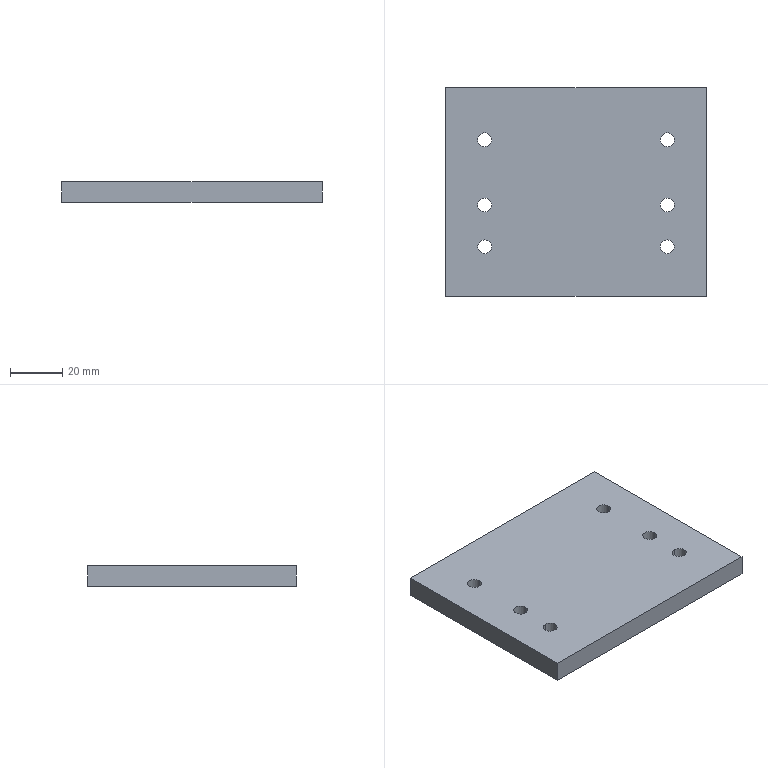Part | SolidWorks | features BaseBody 1 | 1 solid | 18 faces | box 100 x 80 x 8 mm | volume 62941 mm3 | cylinder 12 | plane 6 | commonest cylinder face diameters 5.3 x12
STEP:
#1=CARTESIAN_POINT('',(32.35,20.,-4.));
#2=VERTEX_POINT('',#1);
#3=CARTESIAN_POINT('',(37.65,20.,-4.));
#4=VERTEX_POINT('',#3);
#5=CARTESIAN_POINT('',(35.,20.,-4.));
#6=DIRECTION('',(0.,0.,1.));
#7=DIRECTION('',(1.,0.,0.));
#8=AXIS2_PLACEMENT_3D('',#5,#6,#7);
#9=CIRCLE('',#8,2.65);
#10=EDGE_CURVE('',#2,#4,#9,.T.);
#11=ORIENTED_EDGE('',*,*,#10,.F.);
#12=CARTESIAN_POINT('',(32.35,20.,4.));
#13=VERTEX_POINT('',#12);
#14=CARTESIAN_POINT('',(32.35,20.,-14.2));
#15=DIRECTION('',(0.,0.,1.));
#16=VECTOR('',#15,1000.);
#17=LINE('',#14,#16);
#18=EDGE_CURVE('',#2,#13,#17,.T.);
#19=ORIENTED_EDGE('',*,*,#18,.T.);
#20=CARTESIAN_POINT('',(37.65,20.,4.));
#21=VERTEX_POINT('',#20);
#22=CARTESIAN_POINT('',(35.,20.,4.));
#23=DIRECTION('',(0.,0.,-1.));
#24=DIRECTION('',(1.,0.,0.));
#25=AXIS2_PLACEMENT_3D('',#22,#23,#24);
#26=CIRCLE('',#25,2.65);
#27=EDGE_CURVE('',#21,#13,#26,.T.);
#28=ORIENTED_EDGE('',*,*,#27,.F.);
#29=CARTESIAN_POINT('',(37.65,20.,-14.2));
#30=DIRECTION('',(0.,0.,1.));
#31=VECTOR('',#30,1000.);
#32=LINE('',#29,#31);
#33=EDGE_CURVE('',#4,#21,#32,.T.);
#34=ORIENTED_EDGE('',*,*,#33,.F.);
#35=EDGE_LOOP('',(#11,#19,#28,#34));
#36=FACE_OUTER_BOUND('',#35,.T.);
#37=CARTESIAN_POINT('',(35.,20.,-14.2));
#38=DIRECTION('',(0.,0.,1.));
#39=DIRECTION('',(1.,0.,0.));
#40=AXIS2_PLACEMENT_3D('',#37,#38,#39);
#41=CYLINDRICAL_SURFACE('',#40,2.65);
#42=ADVANCED_FACE('',(#36),#41,.F.);
#43=CARTESIAN_POINT('',(-37.65,20.,-4.));
#44=VERTEX_POINT('',#43);
#45=CARTESIAN_POINT('',(-32.35,20.,-4.));
#46=VERTEX_POINT('',#45);
#47=CARTESIAN_POINT('',(-35.,20.,-4.));
#48=DIRECTION('',(0.,0.,1.));
#49=DIRECTION('',(1.,0.,0.));
#50=AXIS2_PLACEMENT_3D('',#47,#48,#49);
#51=CIRCLE('',#50,2.65);
#52=EDGE_CURVE('',#44,#46,#51,.T.);
#53=ORIENTED_EDGE('',*,*,#52,.F.);
#54=CARTESIAN_POINT('',(-37.65,20.,4.));
#55=VERTEX_POINT('',#54);
#56=CARTESIAN_POINT('',(-37.65,20.,-14.2));
#57=DIRECTION('',(0.,0.,1.));
#58=VECTOR('',#57,1000.);
#59=LINE('',#56,#58);
#60=EDGE_CURVE('',#44,#55,#59,.T.);
#61=ORIENTED_EDGE('',*,*,#60,.T.);
#62=CARTESIAN_POINT('',(-32.35,20.,4.));
#63=VERTEX_POINT('',#62);
#64=CARTESIAN_POINT('',(-35.,20.,4.));
#65=DIRECTION('',(0.,0.,-1.));
#66=DIRECTION('',(1.,0.,0.));
#67=AXIS2_PLACEMENT_3D('',#64,#65,#66);
#68=CIRCLE('',#67,2.65);
#69=EDGE_CURVE('',#63,#55,#68,.T.);
#70=ORIENTED_EDGE('',*,*,#69,.F.);
#71=CARTESIAN_POINT('',(-32.35,20.,-14.2));
#72=DIRECTION('',(0.,0.,1.));
#73=VECTOR('',#72,1000.);
#74=LINE('',#71,#73);
#75=EDGE_CURVE('',#46,#63,#74,.T.);
#76=ORIENTED_EDGE('',*,*,#75,.F.);
#77=EDGE_LOOP('',(#53,#61,#70,#76));
#78=FACE_OUTER_BOUND('',#77,.T.);
#79=CARTESIAN_POINT('',(-35.,20.,-14.2));
#80=DIRECTION('',(0.,0.,1.));
#81=DIRECTION('',(1.,0.,0.));
#82=AXIS2_PLACEMENT_3D('',#79,#80,#81);
#83=CYLINDRICAL_SURFACE('',#82,2.65);
#84=ADVANCED_FACE('',(#78),#83,.F.);
#85=CARTESIAN_POINT('',(32.35,-5.,-4.));
#86=VERTEX_POINT('',#85);
#87=CARTESIAN_POINT('',(37.65,-5.,-4.));
#88=VERTEX_POINT('',#87);
#89=CARTESIAN_POINT('',(35.,-5.,-4.));
#90=DIRECTION('',(0.,0.,1.));
#91=DIRECTION('',(1.,0.,0.));
#92=AXIS2_PLACEMENT_3D('',#89,#90,#91);
#93=CIRCLE('',#92,2.65);
#94=EDGE_CURVE('',#86,#88,#93,.T.);
#95=ORIENTED_EDGE('',*,*,#94,.F.);
#96=CARTESIAN_POINT('',(32.35,-5.,4.));
#97=VERTEX_POINT('',#96);
#98=CARTESIAN_POINT('',(32.35,-5.,-14.2));
#99=DIRECTION('',(0.,0.,1.));
#100=VECTOR('',#99,1000.);
#101=LINE('',#98,#100);
#102=EDGE_CURVE('',#86,#97,#101,.T.);
#103=ORIENTED_EDGE('',*,*,#102,.T.);
#104=CARTESIAN_POINT('',(37.65,-5.,4.));
#105=VERTEX_POINT('',#104);
#106=CARTESIAN_POINT('',(35.,-5.,4.));
#107=DIRECTION('',(0.,0.,-1.));
#108=DIRECTION('',(1.,0.,0.));
#109=AXIS2_PLACEMENT_3D('',#106,#107,#108);
#110=CIRCLE('',#109,2.65);
#111=EDGE_CURVE('',#105,#97,#110,.T.);
#112=ORIENTED_EDGE('',*,*,#111,.F.);
#113=CARTESIAN_POINT('',(37.65,-5.,-14.2));
#114=DIRECTION('',(0.,0.,1.));
#115=VECTOR('',#114,1000.);
#116=LINE('',#113,#115);
#117=EDGE_CURVE('',#88,#105,#116,.T.);
#118=ORIENTED_EDGE('',*,*,#117,.F.);
#119=EDGE_LOOP('',(#95,#103,#112,#118));
#120=FACE_OUTER_BOUND('',#119,.T.);
#121=CARTESIAN_POINT('',(35.,-5.,-14.2));
#122=DIRECTION('',(0.,0.,1.));
#123=DIRECTION('',(1.,0.,0.));
#124=AXIS2_PLACEMENT_3D('',#121,#122,#123);
#125=CYLINDRICAL_SURFACE('',#124,2.65);
#126=ADVANCED_FACE('',(#120),#125,.F.);
#127=CARTESIAN_POINT('',(35.,-23.65,4.));
#128=VERTEX_POINT('',#127);
#129=CARTESIAN_POINT('',(35.,-18.35,4.));
#130=VERTEX_POINT('',#129);
#131=CARTESIAN_POINT('',(35.,-21.,4.));
#132=DIRECTION('',(0.,0.,-1.));
#133=DIRECTION('',(0.,1.,0.));
#134=AXIS2_PLACEMENT_3D('',#131,#132,#133);
#135=CIRCLE('',#134,2.65);
#136=EDGE_CURVE('',#128,#130,#135,.T.);
#137=ORIENTED_EDGE('',*,*,#136,.F.);
#138=CARTESIAN_POINT('',(35.,-23.65,-4.));
#139=VERTEX_POINT('',#138);
#140=CARTESIAN_POINT('',(35.,-23.65,14.2));
#141=DIRECTION('',(0.,0.,-1.));
#142=VECTOR('',#141,1000.);
#143=LINE('',#140,#142);
#144=EDGE_CURVE('',#128,#139,#143,.T.);
#145=ORIENTED_EDGE('',*,*,#144,.T.);
#146=CARTESIAN_POINT('',(35.,-18.35,-4.));
#147=VERTEX_POINT('',#146);
#148=CARTESIAN_POINT('',(35.,-21.,-4.));
#149=DIRECTION('',(0.,0.,1.));
#150=DIRECTION('',(0.,1.,0.));
#151=AXIS2_PLACEMENT_3D('',#148,#149,#150);
#152=CIRCLE('',#151,2.65);
#153=EDGE_CURVE('',#147,#139,#152,.T.);
#154=ORIENTED_EDGE('',*,*,#153,.F.);
#155=CARTESIAN_POINT('',(35.,-18.35,14.2));
#156=DIRECTION('',(0.,0.,-1.));
#157=VECTOR('',#156,1000.);
#158=LINE('',#155,#157);
#159=EDGE_CURVE('',#130,#147,#158,.T.);
#160=ORIENTED_EDGE('',*,*,#159,.F.);
#161=EDGE_LOOP('',(#137,#145,#154,#160));
#162=FACE_OUTER_BOUND('',#161,.T.);
#163=CARTESIAN_POINT('',(35.,-21.,14.2));
#164=DIRECTION('',(0.,0.,-1.));
#165=DIRECTION('',(0.,1.,0.));
#166=AXIS2_PLACEMENT_3D('',#163,#164,#165);
#167=CYLINDRICAL_SURFACE('',#166,2.65);
#168=ADVANCED_FACE('',(#162),#167,.F.);
#169=CARTESIAN_POINT('',(-37.65,-5.,-4.));
#170=VERTEX_POINT('',#169);
#171=CARTESIAN_POINT('',(-32.35,-5.,-4.));
#172=VERTEX_POINT('',#171);
#173=CARTESIAN_POINT('',(-35.,-5.,-4.));
#174=DIRECTION('',(0.,0.,1.));
#175=DIRECTION('',(1.,0.,0.));
#176=AXIS2_PLACEMENT_3D('',#173,#174,#175);
#177=CIRCLE('',#176,2.65);
#178=EDGE_CURVE('',#170,#172,#177,.T.);
#179=ORIENTED_EDGE('',*,*,#178,.F.);
#180=CARTESIAN_POINT('',(-37.65,-5.,4.));
#181=VERTEX_POINT('',#180);
#182=CARTESIAN_POINT('',(-37.65,-5.,-14.2));
#183=DIRECTION('',(0.,0.,1.));
#184=VECTOR('',#183,1000.);
#185=LINE('',#182,#184);
#186=EDGE_CURVE('',#170,#181,#185,.T.);
#187=ORIENTED_EDGE('',*,*,#186,.T.);
#188=CARTESIAN_POINT('',(-32.35,-5.,4.));
#189=VERTEX_POINT('',#188);
#190=CARTESIAN_POINT('',(-35.,-5.,4.));
#191=DIRECTION('',(0.,0.,-1.));
#192=DIRECTION('',(1.,0.,0.));
#193=AXIS2_PLACEMENT_3D('',#190,#191,#192);
#194=CIRCLE('',#193,2.65);
#195=EDGE_CURVE('',#189,#181,#194,.T.);
#196=ORIENTED_EDGE('',*,*,#195,.F.);
#197=CARTESIAN_POINT('',(-32.35,-5.,-14.2));
#198=DIRECTION('',(0.,0.,1.));
#199=VECTOR('',#198,1000.);
#200=LINE('',#197,#199);
#201=EDGE_CURVE('',#172,#189,#200,.T.);
#202=ORIENTED_EDGE('',*,*,#201,.F.);
#203=EDGE_LOOP('',(#179,#187,#196,#202));
#204=FACE_OUTER_BOUND('',#203,.T.);
#205=CARTESIAN_POINT('',(-35.,-5.,-14.2));
#206=DIRECTION('',(0.,0.,1.));
#207=DIRECTION('',(1.,0.,0.));
#208=AXIS2_PLACEMENT_3D('',#205,#206,#207);
#209=CYLINDRICAL_SURFACE('',#208,2.65);
#210=ADVANCED_FACE('',(#204),#209,.F.);
#211=CARTESIAN_POINT('',(-35.,-23.65,4.));
#212=VERTEX_POINT('',#211);
#213=CARTESIAN_POINT('',(-35.,-18.35,4.));
#214=VERTEX_POINT('',#213);
#215=CARTESIAN_POINT('',(-35.,-21.,4.));
#216=DIRECTION('',(0.,0.,-1.));
#217=DIRECTION('',(0.,1.,0.));
#218=AXIS2_PLACEMENT_3D('',#215,#216,#217);
#219=CIRCLE('',#218,2.65);
#220=EDGE_CURVE('',#212,#214,#219,.T.);
#221=ORIENTED_EDGE('',*,*,#220,.F.);
#222=CARTESIAN_POINT('',(-35.,-23.65,-4.));
#223=VERTEX_POINT('',#222);
#224=CARTESIAN_POINT('',(-35.,-23.65,14.2));
#225=DIRECTION('',(0.,0.,-1.));
#226=VECTOR('',#225,1000.);
#227=LINE('',#224,#226);
#228=EDGE_CURVE('',#212,#223,#227,.T.);
#229=ORIENTED_EDGE('',*,*,#228,.T.);
#230=CARTESIAN_POINT('',(-35.,-18.35,-4.));
#231=VERTEX_POINT('',#230);
#232=CARTESIAN_POINT('',(-35.,-21.,-4.));
#233=DIRECTION('',(0.,0.,1.));
#234=DIRECTION('',(0.,1.,0.));
#235=AXIS2_PLACEMENT_3D('',#232,#233,#234);
#236=CIRCLE('',#235,2.65);
#237=EDGE_CURVE('',#231,#223,#236,.T.);
#238=ORIENTED_EDGE('',*,*,#237,.F.);
#239=CARTESIAN_POINT('',(-35.,-18.35,14.2));
#240=DIRECTION('',(0.,0.,-1.));
#241=VECTOR('',#240,1000.);
#242=LINE('',#239,#241);
#243=EDGE_CURVE('',#214,#231,#242,.T.);
#244=ORIENTED_EDGE('',*,*,#243,.F.);
#245=EDGE_LOOP('',(#221,#229,#238,#244));
#246=FACE_OUTER_BOUND('',#245,.T.);
#247=CARTESIAN_POINT('',(-35.,-21.,14.2));
#248=DIRECTION('',(0.,0.,-1.));
#249=DIRECTION('',(0.,1.,0.));
#250=AXIS2_PLACEMENT_3D('',#247,#248,#249);
#251=CYLINDRICAL_SURFACE('',#250,2.65);
#252=ADVANCED_FACE('',(#246),#251,.F.);
#253=ORIENTED_EDGE('',*,*,#27,.T.);
#254=CARTESIAN_POINT('',(35.,20.,4.));
#255=DIRECTION('',(0.,0.,-1.));
#256=DIRECTION('',(1.,0.,0.));
#257=AXIS2_PLACEMENT_3D('',#254,#255,#256);
#258=CIRCLE('',#257,2.65);
#259=EDGE_CURVE('',#13,#21,#258,.T.);
#260=ORIENTED_EDGE('',*,*,#259,.T.);
#261=EDGE_LOOP('',(#253,#260));
#262=FACE_BOUND('',#261,.T.);
#263=ORIENTED_EDGE('',*,*,#69,.T.);
#264=CARTESIAN_POINT('',(-35.,20.,4.));
#265=DIRECTION('',(0.,0.,-1.));
#266=DIRECTION('',(1.,0.,0.));
#267=AXIS2_PLACEMENT_3D('',#264,#265,#266);
#268=CIRCLE('',#267,2.65);
#269=EDGE_CURVE('',#55,#63,#268,.T.);
#270=ORIENTED_EDGE('',*,*,#269,.T.);
#271=EDGE_LOOP('',(#263,#270));
#272=FACE_BOUND('',#271,.T.);
#273=ORIENTED_EDGE('',*,*,#111,.T.);
#274=CARTESIAN_POINT('',(35.,-5.,4.));
#275=DIRECTION('',(0.,0.,-1.));
#276=DIRECTION('',(1.,0.,0.));
#277=AXIS2_PLACEMENT_3D('',#274,#275,#276);
#278=CIRCLE('',#277,2.65);
#279=EDGE_CURVE('',#97,#105,#278,.T.);
#280=ORIENTED_EDGE('',*,*,#279,.T.);
#281=EDGE_LOOP('',(#273,#280));
#282=FACE_BOUND('',#281,.T.);
#283=CARTESIAN_POINT('',(35.,-21.,4.));
#284=DIRECTION('',(0.,0.,-1.));
#285=DIRECTION('',(0.,1.,0.));
#286=AXIS2_PLACEMENT_3D('',#283,#284,#285);
#287=CIRCLE('',#286,2.65);
#288=EDGE_CURVE('',#130,#128,#287,.T.);
#289=ORIENTED_EDGE('',*,*,#288,.T.);
#290=ORIENTED_EDGE('',*,*,#136,.T.);
#291=EDGE_LOOP('',(#289,#290));
#292=FACE_BOUND('',#291,.T.);
#293=ORIENTED_EDGE('',*,*,#195,.T.);
#294=CARTESIAN_POINT('',(-35.,-5.,4.));
#295=DIRECTION('',(0.,0.,-1.));
#296=DIRECTION('',(1.,0.,0.));
#297=AXIS2_PLACEMENT_3D('',#294,#295,#296);
#298=CIRCLE('',#297,2.65);
#299=EDGE_CURVE('',#181,#189,#298,.T.);
#300=ORIENTED_EDGE('',*,*,#299,.T.);
#301=EDGE_LOOP('',(#293,#300));
#302=FACE_BOUND('',#301,.T.);
#303=CARTESIAN_POINT('',(-35.,-21.,4.));
#304=DIRECTION('',(0.,0.,-1.));
#305=DIRECTION('',(0.,1.,0.));
#306=AXIS2_PLACEMENT_3D('',#303,#304,#305);
#307=CIRCLE('',#306,2.65);
#308=EDGE_CURVE('',#214,#212,#307,.T.);
#309=ORIENTED_EDGE('',*,*,#308,.T.);
#310=ORIENTED_EDGE('',*,*,#220,.T.);
#311=EDGE_LOOP('',(#309,#310));
#312=FACE_BOUND('',#311,.T.);
#313=CARTESIAN_POINT('',(50.,-40.,4.));
#314=VERTEX_POINT('',#313);
#315=CARTESIAN_POINT('',(50.,40.,4.));
#316=VERTEX_POINT('',#315);
#317=CARTESIAN_POINT('',(50.,-40.,4.));
#318=DIRECTION('',(0.,1.,0.));
#319=VECTOR('',#318,1000.);
#320=LINE('',#317,#319);
#321=EDGE_CURVE('',#314,#316,#320,.T.);
#322=ORIENTED_EDGE('',*,*,#321,.T.);
#323=CARTESIAN_POINT('',(-50.,40.,4.));
#324=VERTEX_POINT('',#323);
#325=CARTESIAN_POINT('',(-50.,40.,4.));
#326=DIRECTION('',(-1.,0.,0.));
#327=VECTOR('',#326,1000.);
#328=LINE('',#325,#327);
#329=EDGE_CURVE('',#316,#324,#328,.T.);
#330=ORIENTED_EDGE('',*,*,#329,.T.);
#331=CARTESIAN_POINT('',(-50.,-40.,4.));
#332=VERTEX_POINT('',#331);
#333=CARTESIAN_POINT('',(-50.,-40.,4.));
#334=DIRECTION('',(0.,-1.,0.));
#335=VECTOR('',#334,1000.);
#336=LINE('',#333,#335);
#337=EDGE_CURVE('',#324,#332,#336,.T.);
#338=ORIENTED_EDGE('',*,*,#337,.T.);
#339=CARTESIAN_POINT('',(-50.,-40.,4.));
#340=DIRECTION('',(1.,0.,0.));
#341=VECTOR('',#340,1000.);
#342=LINE('',#339,#341);
#343=EDGE_CURVE('',#332,#314,#342,.T.);
#344=ORIENTED_EDGE('',*,*,#343,.T.);
#345=EDGE_LOOP('',(#322,#330,#338,#344));
#346=FACE_OUTER_BOUND('',#345,.T.);
#347=CARTESIAN_POINT('',(-50.,-40.,4.));
#348=DIRECTION('',(0.,0.,1.));
#349=DIRECTION('',(1.,0.,0.));
#350=AXIS2_PLACEMENT_3D('',#347,#348,#349);
#351=PLANE('',#350);
#352=ADVANCED_FACE('',(#262,#272,#282,#292,#302,#312,#346),#351,.T.);
#353=ORIENTED_EDGE('',*,*,#18,.F.);
#354=CARTESIAN_POINT('',(35.,20.,-4.));
#355=DIRECTION('',(0.,0.,1.));
#356=DIRECTION('',(1.,0.,0.));
#357=AXIS2_PLACEMENT_3D('',#354,#355,#356);
#358=CIRCLE('',#357,2.65);
#359=EDGE_CURVE('',#4,#2,#358,.T.);
#360=ORIENTED_EDGE('',*,*,#359,.F.);
#361=ORIENTED_EDGE('',*,*,#33,.T.);
#362=ORIENTED_EDGE('',*,*,#259,.F.);
#363=EDGE_LOOP('',(#353,#360,#361,#362));
#364=FACE_OUTER_BOUND('',#363,.T.);
#365=CARTESIAN_POINT('',(35.,20.,-14.2));
#366=DIRECTION('',(0.,0.,1.));
#367=DIRECTION('',(1.,0.,0.));
#368=AXIS2_PLACEMENT_3D('',#365,#366,#367);
#369=CYLINDRICAL_SURFACE('',#368,2.65);
#370=ADVANCED_FACE('',(#364),#369,.F.);
#371=ORIENTED_EDGE('',*,*,#60,.F.);
#372=CARTESIAN_POINT('',(-35.,20.,-4.));
#373=DIRECTION('',(0.,0.,1.));
#374=DIRECTION('',(1.,0.,0.));
#375=AXIS2_PLACEMENT_3D('',#372,#373,#374);
#376=CIRCLE('',#375,2.65);
#377=EDGE_CURVE('',#46,#44,#376,.T.);
#378=ORIENTED_EDGE('',*,*,#377,.F.);
#379=ORIENTED_EDGE('',*,*,#75,.T.);
#380=ORIENTED_EDGE('',*,*,#269,.F.);
#381=EDGE_LOOP('',(#371,#378,#379,#380));
#382=FACE_OUTER_BOUND('',#381,.T.);
#383=CARTESIAN_POINT('',(-35.,20.,-14.2));
#384=DIRECTION('',(0.,0.,1.));
#385=DIRECTION('',(1.,0.,0.));
#386=AXIS2_PLACEMENT_3D('',#383,#384,#385);
#387=CYLINDRICAL_SURFACE('',#386,2.65);
#388=ADVANCED_FACE('',(#382),#387,.F.);
#389=ORIENTED_EDGE('',*,*,#102,.F.);
#390=CARTESIAN_POINT('',(35.,-5.,-4.));
#391=DIRECTION('',(0.,0.,1.));
#392=DIRECTION('',(1.,0.,0.));
#393=AXIS2_PLACEMENT_3D('',#390,#391,#392);
#394=CIRCLE('',#393,2.65);
#395=EDGE_CURVE('',#88,#86,#394,.T.);
#396=ORIENTED_EDGE('',*,*,#395,.F.);
#397=ORIENTED_EDGE('',*,*,#117,.T.);
#398=ORIENTED_EDGE('',*,*,#279,.F.);
#399=EDGE_LOOP('',(#389,#396,#397,#398));
#400=FACE_OUTER_BOUND('',#399,.T.);
#401=CARTESIAN_POINT('',(35.,-5.,-14.2));
#402=DIRECTION('',(0.,0.,1.));
#403=DIRECTION('',(1.,0.,0.));
#404=AXIS2_PLACEMENT_3D('',#401,#402,#403);
#405=CYLINDRICAL_SURFACE('',#404,2.65);
#406=ADVANCED_FACE('',(#400),#405,.F.);
#407=ORIENTED_EDGE('',*,*,#144,.F.);
#408=ORIENTED_EDGE('',*,*,#288,.F.);
#409=ORIENTED_EDGE('',*,*,#159,.T.);
#410=CARTESIAN_POINT('',(35.,-21.,-4.));
#411=DIRECTION('',(0.,0.,1.));
#412=DIRECTION('',(0.,1.,0.));
#413=AXIS2_PLACEMENT_3D('',#410,#411,#412);
#414=CIRCLE('',#413,2.65);
#415=EDGE_CURVE('',#139,#147,#414,.T.);
#416=ORIENTED_EDGE('',*,*,#415,.F.);
#417=EDGE_LOOP('',(#407,#408,#409,#416));
#418=FACE_OUTER_BOUND('',#417,.T.);
#419=CARTESIAN_POINT('',(35.,-21.,14.2));
#420=DIRECTION('',(0.,0.,-1.));
#421=DIRECTION('',(0.,1.,0.));
#422=AXIS2_PLACEMENT_3D('',#419,#420,#421);
#423=CYLINDRICAL_SURFACE('',#422,2.65);
#424=ADVANCED_FACE('',(#418),#423,.F.);
#425=ORIENTED_EDGE('',*,*,#186,.F.);
#426=CARTESIAN_POINT('',(-35.,-5.,-4.));
#427=DIRECTION('',(0.,0.,1.));
#428=DIRECTION('',(1.,0.,0.));
#429=AXIS2_PLACEMENT_3D('',#426,#427,#428);
#430=CIRCLE('',#429,2.65);
#431=EDGE_CURVE('',#172,#170,#430,.T.);
#432=ORIENTED_EDGE('',*,*,#431,.F.);
#433=ORIENTED_EDGE('',*,*,#201,.T.);
#434=ORIENTED_EDGE('',*,*,#299,.F.);
#435=EDGE_LOOP('',(#425,#432,#433,#434));
#436=FACE_OUTER_BOUND('',#435,.T.);
#437=CARTESIAN_POINT('',(-35.,-5.,-14.2));
#438=DIRECTION('',(0.,0.,1.));
#439=DIRECTION('',(1.,0.,0.));
#440=AXIS2_PLACEMENT_3D('',#437,#438,#439);
#441=CYLINDRICAL_SURFACE('',#440,2.65);
#442=ADVANCED_FACE('',(#436),#441,.F.);
#443=ORIENTED_EDGE('',*,*,#228,.F.);
#444=ORIENTED_EDGE('',*,*,#308,.F.);
#445=ORIENTED_EDGE('',*,*,#243,.T.);
#446=CARTESIAN_POINT('',(-35.,-21.,-4.));
#447=DIRECTION('',(0.,0.,1.));
#448=DIRECTION('',(0.,1.,0.));
#449=AXIS2_PLACEMENT_3D('',#446,#447,#448);
#450=CIRCLE('',#449,2.65);
#451=EDGE_CURVE('',#223,#231,#450,.T.);
#452=ORIENTED_EDGE('',*,*,#451,.F.);
#453=EDGE_LOOP('',(#443,#444,#445,#452));
#454=FACE_OUTER_BOUND('',#453,.T.);
#455=CARTESIAN_POINT('',(-35.,-21.,14.2));
#456=DIRECTION('',(0.,0.,-1.));
#457=DIRECTION('',(0.,1.,0.));
#458=AXIS2_PLACEMENT_3D('',#455,#456,#457);
#459=CYLINDRICAL_SURFACE('',#458,2.65);
#460=ADVANCED_FACE('',(#454),#459,.F.);
#461=ORIENTED_EDGE('',*,*,#329,.F.);
#462=CARTESIAN_POINT('',(50.,40.,-4.));
#463=VERTEX_POINT('',#462);
#464=CARTESIAN_POINT('',(50.,40.,-4.));
#465=DIRECTION('',(0.,0.,-1.));
#466=VECTOR('',#465,1000.);
#467=LINE('',#464,#466);
#468=EDGE_CURVE('',#316,#463,#467,.T.);
#469=ORIENTED_EDGE('',*,*,#468,.T.);
#470=CARTESIAN_POINT('',(-50.,40.,-4.));
#471=VERTEX_POINT('',#470);
#472=CARTESIAN_POINT('',(-50.,40.,-4.));
#473=DIRECTION('',(-1.,0.,0.));
#474=VECTOR('',#473,1000.);
#475=LINE('',#472,#474);
#476=EDGE_CURVE('',#463,#471,#475,.T.);
#477=ORIENTED_EDGE('',*,*,#476,.T.);
#478=CARTESIAN_POINT('',(-50.,40.,-4.));
#479=DIRECTION('',(0.,0.,1.));
#480=VECTOR('',#479,1000.);
#481=LINE('',#478,#480);
#482=EDGE_CURVE('',#471,#324,#481,.T.);
#483=ORIENTED_EDGE('',*,*,#482,.T.);
#484=EDGE_LOOP('',(#461,#469,#477,#483));
#485=FACE_OUTER_BOUND('',#484,.T.);
#486=CARTESIAN_POINT('',(-50.,40.,-4.));
#487=DIRECTION('',(0.,1.,0.));
#488=DIRECTION('',(0.,0.,1.));
#489=AXIS2_PLACEMENT_3D('',#486,#487,#488);
#490=PLANE('',#489);
#491=ADVANCED_FACE('',(#485),#490,.T.);
#492=ORIENTED_EDGE('',*,*,#468,.F.);
#493=ORIENTED_EDGE('',*,*,#321,.F.);
#494=CARTESIAN_POINT('',(50.,-40.,-4.));
#495=VERTEX_POINT('',#494);
#496=CARTESIAN_POINT('',(50.,-40.,-4.));
#497=DIRECTION('',(0.,0.,-1.));
#498=VECTOR('',#497,1000.);
#499=LINE('',#496,#498);
#500=EDGE_CURVE('',#314,#495,#499,.T.);
#501=ORIENTED_EDGE('',*,*,#500,.T.);
#502=CARTESIAN_POINT('',(50.,-40.,-4.));
#503=DIRECTION('',(0.,1.,0.));
#504=VECTOR('',#503,1000.);
#505=LINE('',#502,#504);
#506=EDGE_CURVE('',#495,#463,#505,.T.);
#507=ORIENTED_EDGE('',*,*,#506,.T.);
#508=EDGE_LOOP('',(#492,#493,#501,#507));
#509=FACE_OUTER_BOUND('',#508,.T.);
#510=CARTESIAN_POINT('',(50.,-40.,-4.));
#511=DIRECTION('',(1.,0.,0.));
#512=DIRECTION('',(0.,0.,-1.));
#513=AXIS2_PLACEMENT_3D('',#510,#511,#512);
#514=PLANE('',#513);
#515=ADVANCED_FACE('',(#509),#514,.T.);
#516=ORIENTED_EDGE('',*,*,#343,.F.);
#517=CARTESIAN_POINT('',(-50.,-40.,-4.));
#518=VERTEX_POINT('',#517);
#519=CARTESIAN_POINT('',(-50.,-40.,-4.));
#520=DIRECTION('',(0.,0.,1.));
#521=VECTOR('',#520,1000.);
#522=LINE('',#519,#521);
#523=EDGE_CURVE('',#518,#332,#522,.T.);
#524=ORIENTED_EDGE('',*,*,#523,.F.);
#525=CARTESIAN_POINT('',(-50.,-40.,-4.));
#526=DIRECTION('',(-1.,0.,0.));
#527=VECTOR('',#526,1000.);
#528=LINE('',#525,#527);
#529=EDGE_CURVE('',#495,#518,#528,.T.);
#530=ORIENTED_EDGE('',*,*,#529,.F.);
#531=ORIENTED_EDGE('',*,*,#500,.F.);
#532=EDGE_LOOP('',(#516,#524,#530,#531));
#533=FACE_OUTER_BOUND('',#532,.T.);
#534=CARTESIAN_POINT('',(-50.,-40.,-4.));
#535=DIRECTION('',(0.,1.,0.));
#536=DIRECTION('',(0.,0.,1.));
#537=AXIS2_PLACEMENT_3D('',#534,#535,#536);
#538=PLANE('',#537);
#539=ADVANCED_FACE('',(#533),#538,.F.);
#540=ORIENTED_EDGE('',*,*,#482,.F.);
#541=CARTESIAN_POINT('',(-50.,-40.,-4.));
#542=DIRECTION('',(0.,1.,0.));
#543=VECTOR('',#542,1000.);
#544=LINE('',#541,#543);
#545=EDGE_CURVE('',#518,#471,#544,.T.);
#546=ORIENTED_EDGE('',*,*,#545,.F.);
#547=ORIENTED_EDGE('',*,*,#523,.T.);
#548=ORIENTED_EDGE('',*,*,#337,.F.);
#549=EDGE_LOOP('',(#540,#546,#547,#548));
#550=FACE_OUTER_BOUND('',#549,.T.);
#551=CARTESIAN_POINT('',(-50.,-40.,-4.));
#552=DIRECTION('',(1.,0.,0.));
#553=DIRECTION('',(0.,0.,-1.));
#554=AXIS2_PLACEMENT_3D('',#551,#552,#553);
#555=PLANE('',#554);
#556=ADVANCED_FACE('',(#550),#555,.F.);
#557=ORIENTED_EDGE('',*,*,#359,.T.);
#558=ORIENTED_EDGE('',*,*,#10,.T.);
#559=EDGE_LOOP('',(#557,#558));
#560=FACE_BOUND('',#559,.T.);
#561=ORIENTED_EDGE('',*,*,#377,.T.);
#562=ORIENTED_EDGE('',*,*,#52,.T.);
#563=EDGE_LOOP('',(#561,#562));
#564=FACE_BOUND('',#563,.T.);
#565=ORIENTED_EDGE('',*,*,#395,.T.);
#566=ORIENTED_EDGE('',*,*,#94,.T.);
#567=EDGE_LOOP('',(#565,#566));
#568=FACE_BOUND('',#567,.T.);
#569=ORIENTED_EDGE('',*,*,#153,.T.);
#570=ORIENTED_EDGE('',*,*,#415,.T.);
#571=EDGE_LOOP('',(#569,#570));
#572=FACE_BOUND('',#571,.T.);
#573=ORIENTED_EDGE('',*,*,#431,.T.);
#574=ORIENTED_EDGE('',*,*,#178,.T.);
#575=EDGE_LOOP('',(#573,#574));
#576=FACE_BOUND('',#575,.T.);
#577=ORIENTED_EDGE('',*,*,#237,.T.);
#578=ORIENTED_EDGE('',*,*,#451,.T.);
#579=EDGE_LOOP('',(#577,#578));
#580=FACE_BOUND('',#579,.T.);
#581=ORIENTED_EDGE('',*,*,#506,.F.);
#582=ORIENTED_EDGE('',*,*,#529,.T.);
#583=ORIENTED_EDGE('',*,*,#545,.T.);
#584=ORIENTED_EDGE('',*,*,#476,.F.);
#585=EDGE_LOOP('',(#581,#582,#583,#584));
#586=FACE_OUTER_BOUND('',#585,.T.);
#587=CARTESIAN_POINT('',(-50.,-40.,-4.));
#588=DIRECTION('',(0.,0.,1.));
#589=DIRECTION('',(1.,0.,0.));
#590=AXIS2_PLACEMENT_3D('',#587,#588,#589);
#591=PLANE('',#590);
#592=ADVANCED_FACE('',(#560,#564,#568,#572,#576,#580,#586),#591,.F.);
#593=CLOSED_SHELL('',(#42,#84,#126,#168,#210,#252,#352,#370,#388,#406,#424,#442,#460,#491,#515,#539,#556,#592));
#594=MANIFOLD_SOLID_BREP('',#593);
#595=CARTESIAN_POINT('',(0.,0.,0.));
#596=DIRECTION('',(0.,0.,1.));
#597=DIRECTION('',(1.,0.,0.));
#598=AXIS2_PLACEMENT_3D('',#595,#596,#597);
#599=(LENGTH_UNIT()NAMED_UNIT(*)SI_UNIT(.MILLI.,.METRE.));
#600=UNCERTAINTY_MEASURE_WITH_UNIT(LENGTH_MEASURE(0.00001),#599,'','');
#601=(NAMED_UNIT(*)PLANE_ANGLE_UNIT()SI_UNIT($,.RADIAN.));
#602=(NAMED_UNIT(*)SI_UNIT($,.STERADIAN.)SOLID_ANGLE_UNIT());
#603=(GEOMETRIC_REPRESENTATION_CONTEXT(3)GLOBAL_UNCERTAINTY_ASSIGNED_CONTEXT((#600))GLOBAL_UNIT_ASSIGNED_CONTEXT((#599,#601,#602))REPRESENTATION_CONTEXT('',''));
#604=ADVANCED_BREP_SHAPE_REPRESENTATION('',(#594,#598),#603);